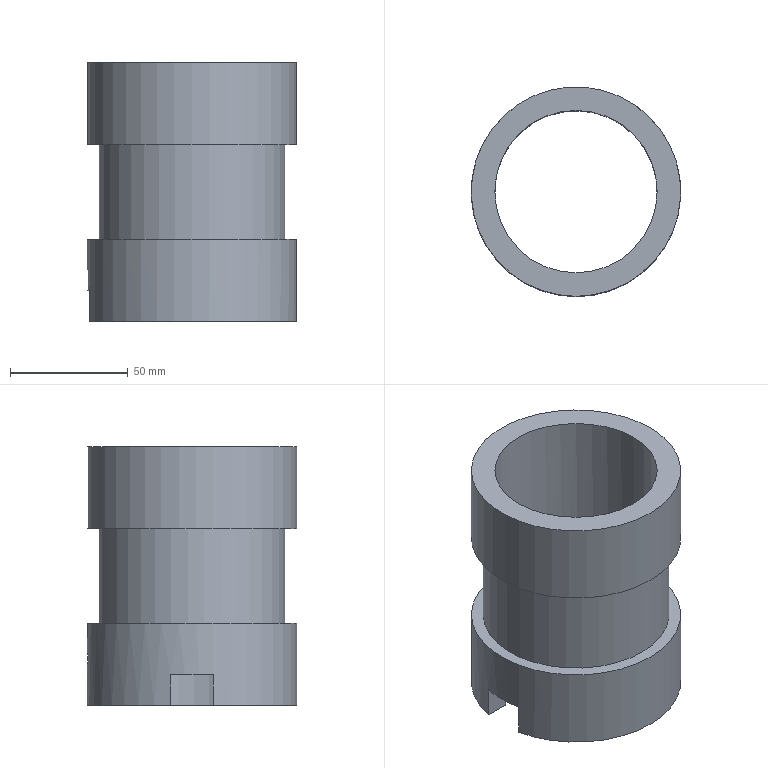Part | NX | features ACO1640-04 2 | 1 solid | 12 faces | box 89 x 89 x 110 mm | volume 217489 mm3 | plane 7 | cylinder 5 | commonest cylinder face diameters 89 x2 6.917 x1 69 x1 79 x1
STEP:
#1=CARTESIAN_POINT('',(1705.554,476.868,18.426));
#2=VERTEX_POINT('',#1);
#3=CARTESIAN_POINT('',(1703.651,476.989,16.352));
#4=CARTESIAN_POINT('',(1705.888,476.848,18.255));
#5=CARTESIAN_POINT('',(1706.12,476.825,21.181));
#6=CARTESIAN_POINT('',(1704.221,476.966,23.411));
#7=CARTESIAN_POINT('',(1701.295,476.989,23.647));
#8=CARTESIAN_POINT('',(1699.062,476.848,21.745));
#9=CARTESIAN_POINT('',(1698.827,476.825,18.824));
#10=CARTESIAN_POINT('',(1700.726,476.966,16.589));
#11=CARTESIAN_POINT('',(1703.651,476.989,16.352));
#12=CARTESIAN_POINT('',(1705.888,476.848,18.255));
#13=CARTESIAN_POINT('',(1706.12,476.825,21.181));
#14=B_SPLINE_CURVE_WITH_KNOTS('',3,(#3,#4,#5,#6,#7,#8,#9,#10,#11,#12,#13),.UNSPECIFIED.,.T.,.F.,(1,1,1,1,1,1,1,1,1,1,1,1,1,1,1),(-0.008112,-0.005408,-0.002704,0.,0.002704,0.005408,0.008112,0.01082,0.01352,0.01622,0.01893,0.02163,0.02434,0.02704,0.02974),.UNSPECIFIED.);
#15=EDGE_CURVE('',#2,#2,#14,.T.);
#16=ORIENTED_EDGE('',*,*,#15,.F.);
#17=EDGE_LOOP('',(#16));
#18=FACE_BOUND('',#17,.T.);
#19=CARTESIAN_POINT('',(1702.673,466.974,16.547));
#20=VERTEX_POINT('',#19);
#21=CARTESIAN_POINT('',(1705.339,466.872,17.453));
#22=CARTESIAN_POINT('',(1702.695,467.017,16.173));
#23=CARTESIAN_POINT('',(1699.924,466.902,17.14));
#24=CARTESIAN_POINT('',(1698.649,466.758,19.776));
#25=CARTESIAN_POINT('',(1699.611,466.872,22.549));
#26=CARTESIAN_POINT('',(1702.253,467.017,23.826));
#27=CARTESIAN_POINT('',(1705.021,466.903,22.864));
#28=CARTESIAN_POINT('',(1706.3,466.758,20.225));
#29=CARTESIAN_POINT('',(1705.339,466.872,17.453));
#30=CARTESIAN_POINT('',(1702.695,467.017,16.173));
#31=CARTESIAN_POINT('',(1699.924,466.902,17.14));
#32=B_SPLINE_CURVE_WITH_KNOTS('',3,(#21,#22,#23,#24,#25,#26,#27,#28,#29,#30,#31),.UNSPECIFIED.,.T.,.F.,(1,1,1,1,1,1,1,1,1,1,1,1,1,1,1),(-0.008114,-0.005409,-0.002705,0.,0.002705,0.005409,0.008114,0.01082,0.01352,0.01623,0.01893,0.02164,0.02434,0.02705,0.02975),.UNSPECIFIED.);
#33=EDGE_CURVE('',#20,#20,#32,.T.);
#34=ORIENTED_EDGE('',*,*,#33,.F.);
#35=EDGE_LOOP('',(#34));
#36=FACE_BOUND('',#35,.T.);
#37=CARTESIAN_POINT('',(1702.474,473.874,20.));
#38=DIRECTION('',(0.,-1.,0.));
#39=DIRECTION('',(-1.,0.,0.));
#40=AXIS2_PLACEMENT_3D('',#37,#38,#39);
#41=CYLINDRICAL_SURFACE('',#40,3.458);
#42=ADVANCED_FACE('',(#18,#36),#41,.F.);
#43=CARTESIAN_POINT('',(1702.474,387.974,35.));
#44=VERTEX_POINT('',#43);
#45=CARTESIAN_POINT('',(1702.474,432.474,35.));
#46=DIRECTION('',(0.,0.,1.));
#47=DIRECTION('',(0.,-1.,0.));
#48=AXIS2_PLACEMENT_3D('',#45,#46,#47);
#49=CIRCLE('',#48,44.5);
#50=EDGE_CURVE('',#44,#44,#49,.T.);
#51=ORIENTED_EDGE('',*,*,#50,.F.);
#52=EDGE_LOOP('',(#51));
#53=FACE_BOUND('',#52,.T.);
#54=CARTESIAN_POINT('',(1658.894,423.474,0.));
#55=VERTEX_POINT('',#54);
#56=CARTESIAN_POINT('',(1658.894,441.474,0.));
#57=VERTEX_POINT('',#56);
#58=CARTESIAN_POINT('',(1702.474,432.474,0.));
#59=DIRECTION('',(0.,0.,1.));
#60=DIRECTION('',(0.,-1.,0.));
#61=AXIS2_PLACEMENT_3D('',#58,#59,#60);
#62=CIRCLE('',#61,44.5);
#63=EDGE_CURVE('',#55,#57,#62,.T.);
#64=ORIENTED_EDGE('',*,*,#63,.T.);
#65=CARTESIAN_POINT('',(1658.894,441.474,13.));
#66=VERTEX_POINT('',#65);
#67=CARTESIAN_POINT('',(1658.894,441.474,6.5));
#68=DIRECTION('',(0.,0.,-1.));
#69=VECTOR('',#68,1000.);
#70=LINE('',#67,#69);
#71=EDGE_CURVE('',#57,#66,#70,.F.);
#72=ORIENTED_EDGE('',*,*,#71,.T.);
#73=CARTESIAN_POINT('',(1658.894,423.474,13.));
#74=VERTEX_POINT('',#73);
#75=CARTESIAN_POINT('',(1702.474,432.474,13.));
#76=DIRECTION('',(0.,0.,-1.));
#77=DIRECTION('',(0.,1.,0.));
#78=AXIS2_PLACEMENT_3D('',#75,#76,#77);
#79=CIRCLE('',#78,44.5);
#80=EDGE_CURVE('',#74,#66,#79,.T.);
#81=ORIENTED_EDGE('',*,*,#80,.F.);
#82=CARTESIAN_POINT('',(1658.894,423.474,6.5));
#83=DIRECTION('',(0.,0.,-1.));
#84=VECTOR('',#83,1000.);
#85=LINE('',#82,#84);
#86=EDGE_CURVE('',#74,#55,#85,.T.);
#87=ORIENTED_EDGE('',*,*,#86,.T.);
#88=EDGE_LOOP('',(#64,#72,#81,#87));
#89=FACE_BOUND('',#88,.T.);
#90=ORIENTED_EDGE('',*,*,#15,.T.);
#91=EDGE_LOOP('',(#90));
#92=FACE_BOUND('',#91,.T.);
#93=CARTESIAN_POINT('',(1702.474,432.474,82.5));
#94=DIRECTION('',(0.,0.,-1.));
#95=DIRECTION('',(1.,0.,0.));
#96=AXIS2_PLACEMENT_3D('',#93,#94,#95);
#97=CYLINDRICAL_SURFACE('',#96,44.5);
#98=ADVANCED_FACE('',(#53,#89,#92),#97,.T.);
#99=CARTESIAN_POINT('',(1669.169,423.474,0.));
#100=VERTEX_POINT('',#99);
#101=CARTESIAN_POINT('',(1669.169,441.474,0.));
#102=VERTEX_POINT('',#101);
#103=CARTESIAN_POINT('',(1702.474,432.474,0.));
#104=DIRECTION('',(0.,0.,1.));
#105=DIRECTION('',(0.,-1.,0.));
#106=AXIS2_PLACEMENT_3D('',#103,#104,#105);
#107=CIRCLE('',#106,34.5);
#108=EDGE_CURVE('',#100,#102,#107,.T.);
#109=ORIENTED_EDGE('',*,*,#108,.F.);
#110=CARTESIAN_POINT('',(1669.169,423.474,13.));
#111=VERTEX_POINT('',#110);
#112=CARTESIAN_POINT('',(1669.169,423.474,-48.5));
#113=DIRECTION('',(0.,0.,-1.));
#114=VECTOR('',#113,1000.);
#115=LINE('',#112,#114);
#116=EDGE_CURVE('',#100,#111,#115,.F.);
#117=ORIENTED_EDGE('',*,*,#116,.T.);
#118=CARTESIAN_POINT('',(1669.169,441.474,13.));
#119=VERTEX_POINT('',#118);
#120=CARTESIAN_POINT('',(1702.474,432.474,13.));
#121=DIRECTION('',(0.,0.,-1.));
#122=DIRECTION('',(0.,1.,0.));
#123=AXIS2_PLACEMENT_3D('',#120,#121,#122);
#124=CIRCLE('',#123,34.5);
#125=EDGE_CURVE('',#111,#119,#124,.T.);
#126=ORIENTED_EDGE('',*,*,#125,.T.);
#127=CARTESIAN_POINT('',(1669.169,441.474,-48.5));
#128=DIRECTION('',(0.,0.,-1.));
#129=VECTOR('',#128,1000.);
#130=LINE('',#127,#129);
#131=EDGE_CURVE('',#102,#119,#130,.F.);
#132=ORIENTED_EDGE('',*,*,#131,.F.);
#133=EDGE_LOOP('',(#109,#117,#126,#132));
#134=FACE_BOUND('',#133,.T.);
#135=CARTESIAN_POINT('',(1702.474,397.974,110.));
#136=VERTEX_POINT('',#135);
#137=CARTESIAN_POINT('',(1702.474,432.474,110.));
#138=DIRECTION('',(0.,0.,1.));
#139=DIRECTION('',(0.,-1.,0.));
#140=AXIS2_PLACEMENT_3D('',#137,#138,#139);
#141=CIRCLE('',#140,34.5);
#142=EDGE_CURVE('',#136,#136,#141,.T.);
#143=ORIENTED_EDGE('',*,*,#142,.T.);
#144=EDGE_LOOP('',(#143));
#145=FACE_BOUND('',#144,.T.);
#146=ORIENTED_EDGE('',*,*,#33,.T.);
#147=EDGE_LOOP('',(#146));
#148=FACE_BOUND('',#147,.T.);
#149=CARTESIAN_POINT('',(1702.474,432.474,27.5));
#150=DIRECTION('',(0.,0.,-1.));
#151=DIRECTION('',(1.,0.,0.));
#152=AXIS2_PLACEMENT_3D('',#149,#150,#151);
#153=CYLINDRICAL_SURFACE('',#152,34.5);
#154=ADVANCED_FACE('',(#134,#145,#148),#153,.F.);
#155=ORIENTED_EDGE('',*,*,#50,.T.);
#156=EDGE_LOOP('',(#155));
#157=FACE_BOUND('',#156,.T.);
#158=CARTESIAN_POINT('',(1702.474,392.974,35.));
#159=VERTEX_POINT('',#158);
#160=CARTESIAN_POINT('',(1702.474,432.474,35.));
#161=DIRECTION('',(0.,0.,1.));
#162=DIRECTION('',(0.,-1.,0.));
#163=AXIS2_PLACEMENT_3D('',#160,#161,#162);
#164=CIRCLE('',#163,39.5);
#165=EDGE_CURVE('',#159,#159,#164,.T.);
#166=ORIENTED_EDGE('',*,*,#165,.F.);
#167=EDGE_LOOP('',(#166));
#168=FACE_BOUND('',#167,.T.);
#169=CARTESIAN_POINT('',(1702.474,468.974,35.));
#170=DIRECTION('',(0.,0.,-1.));
#171=DIRECTION('',(1.,0.,0.));
#172=AXIS2_PLACEMENT_3D('',#169,#170,#171);
#173=PLANE('',#172);
#174=ADVANCED_FACE('',(#157,#168),#173,.F.);
#175=CARTESIAN_POINT('',(1702.474,392.974,75.));
#176=VERTEX_POINT('',#175);
#177=CARTESIAN_POINT('',(1702.474,432.474,75.));
#178=DIRECTION('',(0.,0.,1.));
#179=DIRECTION('',(0.,-1.,0.));
#180=AXIS2_PLACEMENT_3D('',#177,#178,#179);
#181=CIRCLE('',#180,39.5);
#182=EDGE_CURVE('',#176,#176,#181,.T.);
#183=ORIENTED_EDGE('',*,*,#182,.F.);
#184=EDGE_LOOP('',(#183));
#185=FACE_BOUND('',#184,.T.);
#186=ORIENTED_EDGE('',*,*,#165,.T.);
#187=EDGE_LOOP('',(#186));
#188=FACE_BOUND('',#187,.T.);
#189=CARTESIAN_POINT('',(1702.474,432.474,27.5));
#190=DIRECTION('',(0.,0.,-1.));
#191=DIRECTION('',(1.,0.,0.));
#192=AXIS2_PLACEMENT_3D('',#189,#190,#191);
#193=CYLINDRICAL_SURFACE('',#192,39.5);
#194=ADVANCED_FACE('',(#185,#188),#193,.T.);
#195=CARTESIAN_POINT('',(1702.474,387.974,75.));
#196=VERTEX_POINT('',#195);
#197=CARTESIAN_POINT('',(1702.474,432.474,75.));
#198=DIRECTION('',(0.,0.,1.));
#199=DIRECTION('',(0.,-1.,0.));
#200=AXIS2_PLACEMENT_3D('',#197,#198,#199);
#201=CIRCLE('',#200,44.5);
#202=EDGE_CURVE('',#196,#196,#201,.T.);
#203=ORIENTED_EDGE('',*,*,#202,.F.);
#204=EDGE_LOOP('',(#203));
#205=FACE_BOUND('',#204,.T.);
#206=ORIENTED_EDGE('',*,*,#182,.T.);
#207=EDGE_LOOP('',(#206));
#208=FACE_BOUND('',#207,.T.);
#209=CARTESIAN_POINT('',(1702.474,473.974,75.));
#210=DIRECTION('',(0.,0.,-1.));
#211=DIRECTION('',(1.,0.,0.));
#212=AXIS2_PLACEMENT_3D('',#209,#210,#211);
#213=PLANE('',#212);
#214=ADVANCED_FACE('',(#205,#208),#213,.T.);
#215=CARTESIAN_POINT('',(1702.474,387.974,110.));
#216=VERTEX_POINT('',#215);
#217=CARTESIAN_POINT('',(1702.474,432.474,110.));
#218=DIRECTION('',(0.,0.,1.));
#219=DIRECTION('',(0.,-1.,0.));
#220=AXIS2_PLACEMENT_3D('',#217,#218,#219);
#221=CIRCLE('',#220,44.5);
#222=EDGE_CURVE('',#216,#216,#221,.T.);
#223=ORIENTED_EDGE('',*,*,#222,.F.);
#224=EDGE_LOOP('',(#223));
#225=FACE_BOUND('',#224,.T.);
#226=ORIENTED_EDGE('',*,*,#202,.T.);
#227=EDGE_LOOP('',(#226));
#228=FACE_BOUND('',#227,.T.);
#229=CARTESIAN_POINT('',(1702.474,432.474,27.5));
#230=DIRECTION('',(0.,0.,-1.));
#231=DIRECTION('',(1.,0.,0.));
#232=AXIS2_PLACEMENT_3D('',#229,#230,#231);
#233=CYLINDRICAL_SURFACE('',#232,44.5);
#234=ADVANCED_FACE('',(#225,#228),#233,.T.);
#235=CARTESIAN_POINT('',(1667.125,441.474,13.));
#236=DIRECTION('',(-1.,0.,0.));
#237=VECTOR('',#236,1000.);
#238=LINE('',#235,#237);
#239=EDGE_CURVE('',#119,#66,#238,.T.);
#240=ORIENTED_EDGE('',*,*,#239,.F.);
#241=ORIENTED_EDGE('',*,*,#125,.F.);
#242=CARTESIAN_POINT('',(1667.125,423.474,13.));
#243=DIRECTION('',(-1.,0.,0.));
#244=VECTOR('',#243,1000.);
#245=LINE('',#242,#244);
#246=EDGE_CURVE('',#111,#74,#245,.T.);
#247=ORIENTED_EDGE('',*,*,#246,.T.);
#248=ORIENTED_EDGE('',*,*,#80,.T.);
#249=EDGE_LOOP('',(#240,#241,#247,#248));
#250=FACE_BOUND('',#249,.T.);
#251=CARTESIAN_POINT('',(1702.474,441.474,13.));
#252=DIRECTION('',(0.,0.,1.));
#253=DIRECTION('',(-1.,0.,0.));
#254=AXIS2_PLACEMENT_3D('',#251,#252,#253);
#255=PLANE('',#254);
#256=ADVANCED_FACE('',(#250),#255,.F.);
#257=ORIENTED_EDGE('',*,*,#246,.F.);
#258=ORIENTED_EDGE('',*,*,#116,.F.);
#259=CARTESIAN_POINT('',(1667.125,423.474,0.));
#260=DIRECTION('',(-1.,0.,0.));
#261=VECTOR('',#260,1000.);
#262=LINE('',#259,#261);
#263=EDGE_CURVE('',#100,#55,#262,.T.);
#264=ORIENTED_EDGE('',*,*,#263,.T.);
#265=ORIENTED_EDGE('',*,*,#86,.F.);
#266=EDGE_LOOP('',(#257,#258,#264,#265));
#267=FACE_BOUND('',#266,.T.);
#268=CARTESIAN_POINT('',(1702.474,423.474,13.));
#269=DIRECTION('',(0.,-1.,0.));
#270=DIRECTION('',(0.,0.,-1.));
#271=AXIS2_PLACEMENT_3D('',#268,#269,#270);
#272=PLANE('',#271);
#273=ADVANCED_FACE('',(#267),#272,.F.);
#274=CARTESIAN_POINT('',(1667.125,441.474,0.));
#275=DIRECTION('',(-1.,0.,0.));
#276=VECTOR('',#275,1000.);
#277=LINE('',#274,#276);
#278=EDGE_CURVE('',#102,#57,#277,.T.);
#279=ORIENTED_EDGE('',*,*,#278,.F.);
#280=ORIENTED_EDGE('',*,*,#131,.T.);
#281=ORIENTED_EDGE('',*,*,#239,.T.);
#282=ORIENTED_EDGE('',*,*,#71,.F.);
#283=EDGE_LOOP('',(#279,#280,#281,#282));
#284=FACE_BOUND('',#283,.T.);
#285=CARTESIAN_POINT('',(1702.474,441.474,0.));
#286=DIRECTION('',(0.,1.,0.));
#287=DIRECTION('',(0.,0.,1.));
#288=AXIS2_PLACEMENT_3D('',#285,#286,#287);
#289=PLANE('',#288);
#290=ADVANCED_FACE('',(#284),#289,.F.);
#291=ORIENTED_EDGE('',*,*,#222,.T.);
#292=EDGE_LOOP('',(#291));
#293=FACE_BOUND('',#292,.T.);
#294=ORIENTED_EDGE('',*,*,#142,.F.);
#295=EDGE_LOOP('',(#294));
#296=FACE_BOUND('',#295,.T.);
#297=CARTESIAN_POINT('',(1702.474,463.974,110.));
#298=DIRECTION('',(0.,0.,-1.));
#299=DIRECTION('',(1.,0.,0.));
#300=AXIS2_PLACEMENT_3D('',#297,#298,#299);
#301=PLANE('',#300);
#302=ADVANCED_FACE('',(#293,#296),#301,.F.);
#303=ORIENTED_EDGE('',*,*,#263,.F.);
#304=ORIENTED_EDGE('',*,*,#108,.T.);
#305=ORIENTED_EDGE('',*,*,#278,.T.);
#306=ORIENTED_EDGE('',*,*,#63,.F.);
#307=EDGE_LOOP('',(#303,#304,#305,#306));
#308=FACE_BOUND('',#307,.T.);
#309=CARTESIAN_POINT('',(1702.474,463.974,0.));
#310=DIRECTION('',(0.,0.,-1.));
#311=DIRECTION('',(1.,0.,0.));
#312=AXIS2_PLACEMENT_3D('',#309,#310,#311);
#313=PLANE('',#312);
#314=ADVANCED_FACE('',(#308),#313,.T.);
#315=CLOSED_SHELL('',(#42,#98,#154,#174,#194,#214,#234,#256,#273,#290,#302,#314));
#316=MANIFOLD_SOLID_BREP('',#315);
#317=(LENGTH_UNIT()NAMED_UNIT(*)SI_UNIT(.MILLI.,.METRE.));
#318=UNCERTAINTY_MEASURE_WITH_UNIT(LENGTH_MEASURE(0.0508),#317,'','');
#319=(NAMED_UNIT(*)PLANE_ANGLE_UNIT()SI_UNIT($,.RADIAN.));
#320=(NAMED_UNIT(*)SI_UNIT($,.STERADIAN.)SOLID_ANGLE_UNIT());
#321=(GEOMETRIC_REPRESENTATION_CONTEXT(3)GLOBAL_UNCERTAINTY_ASSIGNED_CONTEXT((#318))GLOBAL_UNIT_ASSIGNED_CONTEXT((#317,#319,#320))REPRESENTATION_CONTEXT('',''));
#322=ADVANCED_BREP_SHAPE_REPRESENTATION('',(#316),#321);